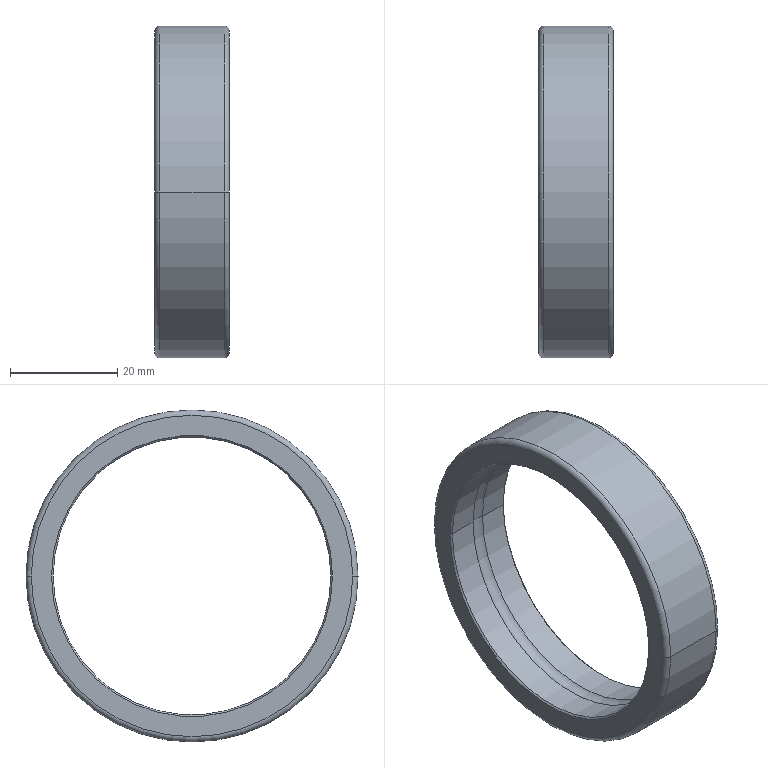Part | SolidWorks | 1 solid | 18 faces | box 14 x 62 x 62 mm | volume 12465 mm3 | cylinder 6 | torus 6 | cone 4 | plane 2 | commonest cylinder face diameters 51.875 x4 62 x2
STEP:
#1=CARTESIAN_POINT('',(0.3,-25.938,0.));
#2=VERTEX_POINT('',#1);
#3=CARTESIAN_POINT('',(0.,-26.238,0.));
#4=VERTEX_POINT('',#3);
#5=CARTESIAN_POINT('',(0.3,-25.938,0.));
#6=DIRECTION('',(-0.7071,-0.7071,0.));
#7=VECTOR('',#6,1000.);
#8=LINE('',#5,#7);
#9=EDGE_CURVE('',#2,#4,#8,.T.);
#10=ORIENTED_EDGE('',*,*,#9,.T.);
#11=CARTESIAN_POINT('',(0.,26.238,0.));
#12=VERTEX_POINT('',#11);
#13=CARTESIAN_POINT('',(0.,0.,0.));
#14=DIRECTION('',(-1.,0.,0.));
#15=DIRECTION('',(0.,-1.,0.));
#16=AXIS2_PLACEMENT_3D('',#13,#14,#15);
#17=CIRCLE('',#16,26.238);
#18=EDGE_CURVE('',#4,#12,#17,.T.);
#19=ORIENTED_EDGE('',*,*,#18,.T.);
#20=CARTESIAN_POINT('',(0.3,25.938,0.));
#21=VERTEX_POINT('',#20);
#22=CARTESIAN_POINT('',(0.3,25.938,0.));
#23=DIRECTION('',(-0.7071,0.7071,0.));
#24=VECTOR('',#23,1000.);
#25=LINE('',#22,#24);
#26=EDGE_CURVE('',#21,#12,#25,.T.);
#27=ORIENTED_EDGE('',*,*,#26,.F.);
#28=CARTESIAN_POINT('',(0.3,0.,0.));
#29=DIRECTION('',(-1.,0.,0.));
#30=DIRECTION('',(0.,-1.,0.));
#31=AXIS2_PLACEMENT_3D('',#28,#29,#30);
#32=CIRCLE('',#31,25.938);
#33=EDGE_CURVE('',#2,#21,#32,.T.);
#34=ORIENTED_EDGE('',*,*,#33,.F.);
#35=EDGE_LOOP('',(#10,#19,#27,#34));
#36=FACE_OUTER_BOUND('',#35,.T.);
#37=CARTESIAN_POINT('',(0.3753,0.,0.));
#38=DIRECTION('',(-1.,0.,0.));
#39=DIRECTION('',(0.,1.,0.));
#40=AXIS2_PLACEMENT_3D('',#37,#38,#39);
#41=CONICAL_SURFACE('',#40,25.862,0.7854);
#42=ADVANCED_FACE('',(#36),#41,.F.);
#43=CARTESIAN_POINT('',(13.7,-25.938,0.));
#44=VERTEX_POINT('',#43);
#45=CARTESIAN_POINT('',(8.25,-25.938,0.));
#46=VERTEX_POINT('',#45);
#47=CARTESIAN_POINT('',(13.7,-25.938,0.));
#48=DIRECTION('',(-1.,0.,0.));
#49=VECTOR('',#48,1000.);
#50=LINE('',#47,#49);
#51=EDGE_CURVE('',#44,#46,#50,.T.);
#52=ORIENTED_EDGE('',*,*,#51,.T.);
#53=CARTESIAN_POINT('',(8.25,25.938,0.));
#54=VERTEX_POINT('',#53);
#55=CARTESIAN_POINT('',(8.25,0.,0.));
#56=DIRECTION('',(-1.,0.,0.));
#57=DIRECTION('',(0.,-1.,0.));
#58=AXIS2_PLACEMENT_3D('',#55,#56,#57);
#59=CIRCLE('',#58,25.938);
#60=EDGE_CURVE('',#46,#54,#59,.T.);
#61=ORIENTED_EDGE('',*,*,#60,.T.);
#62=CARTESIAN_POINT('',(13.7,25.938,0.));
#63=VERTEX_POINT('',#62);
#64=CARTESIAN_POINT('',(13.7,25.938,0.));
#65=DIRECTION('',(-1.,0.,0.));
#66=VECTOR('',#65,1000.);
#67=LINE('',#64,#66);
#68=EDGE_CURVE('',#63,#54,#67,.T.);
#69=ORIENTED_EDGE('',*,*,#68,.F.);
#70=CARTESIAN_POINT('',(13.7,0.,0.));
#71=DIRECTION('',(1.,0.,0.));
#72=DIRECTION('',(0.,1.,0.));
#73=AXIS2_PLACEMENT_3D('',#70,#71,#72);
#74=CIRCLE('',#73,25.938);
#75=EDGE_CURVE('',#63,#44,#74,.T.);
#76=ORIENTED_EDGE('',*,*,#75,.T.);
#77=EDGE_LOOP('',(#52,#61,#69,#76));
#78=FACE_OUTER_BOUND('',#77,.T.);
#79=CARTESIAN_POINT('',(0.,0.,0.));
#80=DIRECTION('',(1.,0.,0.));
#81=DIRECTION('',(0.,-1.,0.));
#82=AXIS2_PLACEMENT_3D('',#79,#80,#81);
#83=CYLINDRICAL_SURFACE('',#82,25.938);
#84=ADVANCED_FACE('',(#78),#83,.F.);
#85=CARTESIAN_POINT('',(5.75,-25.938,0.));
#86=VERTEX_POINT('',#85);
#87=CARTESIAN_POINT('',(7.,-24.25,0.));
#88=DIRECTION('',(0.,0.,-1.));
#89=DIRECTION('',(0.5952,-0.8036,0.));
#90=AXIS2_PLACEMENT_3D('',#87,#88,#89);
#91=CIRCLE('',#90,2.1);
#92=EDGE_CURVE('',#46,#86,#91,.T.);
#93=ORIENTED_EDGE('',*,*,#92,.T.);
#94=CARTESIAN_POINT('',(5.75,25.938,0.));
#95=VERTEX_POINT('',#94);
#96=CARTESIAN_POINT('',(5.75,0.,0.));
#97=DIRECTION('',(1.,0.,0.));
#98=DIRECTION('',(0.,1.,0.));
#99=AXIS2_PLACEMENT_3D('',#96,#97,#98);
#100=CIRCLE('',#99,25.938);
#101=EDGE_CURVE('',#95,#86,#100,.T.);
#102=ORIENTED_EDGE('',*,*,#101,.F.);
#103=CARTESIAN_POINT('',(7.,24.25,0.));
#104=DIRECTION('',(0.,0.,1.));
#105=DIRECTION('',(0.,1.,0.));
#106=AXIS2_PLACEMENT_3D('',#103,#104,#105);
#107=CIRCLE('',#106,2.1);
#108=EDGE_CURVE('',#54,#95,#107,.T.);
#109=ORIENTED_EDGE('',*,*,#108,.F.);
#110=ORIENTED_EDGE('',*,*,#60,.F.);
#111=EDGE_LOOP('',(#93,#102,#109,#110));
#112=FACE_OUTER_BOUND('',#111,.T.);
#113=CARTESIAN_POINT('',(7.,0.,0.));
#114=DIRECTION('',(1.,0.,0.));
#115=DIRECTION('',(0.,-1.,0.));
#116=AXIS2_PLACEMENT_3D('',#113,#114,#115);
#117=TOROIDAL_SURFACE('',#116,24.25,2.1);
#118=ADVANCED_FACE('',(#112),#117,.F.);
#119=CARTESIAN_POINT('',(5.75,-25.938,0.));
#120=DIRECTION('',(-1.,0.,0.));
#121=VECTOR('',#120,1000.);
#122=LINE('',#119,#121);
#123=EDGE_CURVE('',#86,#2,#122,.T.);
#124=ORIENTED_EDGE('',*,*,#123,.T.);
#125=ORIENTED_EDGE('',*,*,#33,.T.);
#126=CARTESIAN_POINT('',(5.75,25.938,0.));
#127=DIRECTION('',(-1.,0.,0.));
#128=VECTOR('',#127,1000.);
#129=LINE('',#126,#128);
#130=EDGE_CURVE('',#95,#21,#129,.T.);
#131=ORIENTED_EDGE('',*,*,#130,.F.);
#132=ORIENTED_EDGE('',*,*,#101,.T.);
#133=EDGE_LOOP('',(#124,#125,#131,#132));
#134=FACE_OUTER_BOUND('',#133,.T.);
#135=CARTESIAN_POINT('',(0.,0.,0.));
#136=DIRECTION('',(1.,0.,0.));
#137=DIRECTION('',(0.,-1.,0.));
#138=AXIS2_PLACEMENT_3D('',#135,#136,#137);
#139=CYLINDRICAL_SURFACE('',#138,25.938);
#140=ADVANCED_FACE('',(#134),#139,.F.);
#141=ORIENTED_EDGE('',*,*,#123,.F.);
#142=CARTESIAN_POINT('',(5.75,0.,0.));
#143=DIRECTION('',(1.,0.,0.));
#144=DIRECTION('',(0.,-1.,0.));
#145=AXIS2_PLACEMENT_3D('',#142,#143,#144);
#146=CIRCLE('',#145,25.938);
#147=EDGE_CURVE('',#86,#95,#146,.T.);
#148=ORIENTED_EDGE('',*,*,#147,.T.);
#149=ORIENTED_EDGE('',*,*,#130,.T.);
#150=CARTESIAN_POINT('',(0.3,0.,0.));
#151=DIRECTION('',(-1.,0.,0.));
#152=DIRECTION('',(0.,1.,0.));
#153=AXIS2_PLACEMENT_3D('',#150,#151,#152);
#154=CIRCLE('',#153,25.938);
#155=EDGE_CURVE('',#21,#2,#154,.T.);
#156=ORIENTED_EDGE('',*,*,#155,.T.);
#157=EDGE_LOOP('',(#141,#148,#149,#156));
#158=FACE_OUTER_BOUND('',#157,.T.);
#159=CARTESIAN_POINT('',(0.,0.,0.));
#160=DIRECTION('',(1.,0.,0.));
#161=DIRECTION('',(0.,-1.,0.));
#162=AXIS2_PLACEMENT_3D('',#159,#160,#161);
#163=CYLINDRICAL_SURFACE('',#162,25.938);
#164=ADVANCED_FACE('',(#158),#163,.F.);
#165=ORIENTED_EDGE('',*,*,#147,.F.);
#166=ORIENTED_EDGE('',*,*,#92,.F.);
#167=CARTESIAN_POINT('',(8.25,0.,0.));
#168=DIRECTION('',(-1.,0.,0.));
#169=DIRECTION('',(0.,1.,0.));
#170=AXIS2_PLACEMENT_3D('',#167,#168,#169);
#171=CIRCLE('',#170,25.938);
#172=EDGE_CURVE('',#54,#46,#171,.T.);
#173=ORIENTED_EDGE('',*,*,#172,.F.);
#174=ORIENTED_EDGE('',*,*,#108,.T.);
#175=EDGE_LOOP('',(#165,#166,#173,#174));
#176=FACE_OUTER_BOUND('',#175,.T.);
#177=CARTESIAN_POINT('',(7.,0.,0.));
#178=DIRECTION('',(1.,0.,0.));
#179=DIRECTION('',(0.,-1.,0.));
#180=AXIS2_PLACEMENT_3D('',#177,#178,#179);
#181=TOROIDAL_SURFACE('',#180,24.25,2.1);
#182=ADVANCED_FACE('',(#176),#181,.F.);
#183=ORIENTED_EDGE('',*,*,#51,.F.);
#184=CARTESIAN_POINT('',(13.7,0.,0.));
#185=DIRECTION('',(1.,0.,0.));
#186=DIRECTION('',(0.,-1.,0.));
#187=AXIS2_PLACEMENT_3D('',#184,#185,#186);
#188=CIRCLE('',#187,25.938);
#189=EDGE_CURVE('',#44,#63,#188,.T.);
#190=ORIENTED_EDGE('',*,*,#189,.T.);
#191=ORIENTED_EDGE('',*,*,#68,.T.);
#192=ORIENTED_EDGE('',*,*,#172,.T.);
#193=EDGE_LOOP('',(#183,#190,#191,#192));
#194=FACE_OUTER_BOUND('',#193,.T.);
#195=CARTESIAN_POINT('',(0.,0.,0.));
#196=DIRECTION('',(1.,0.,0.));
#197=DIRECTION('',(0.,-1.,0.));
#198=AXIS2_PLACEMENT_3D('',#195,#196,#197);
#199=CYLINDRICAL_SURFACE('',#198,25.938);
#200=ADVANCED_FACE('',(#194),#199,.F.);
#201=CARTESIAN_POINT('',(14.,-26.238,0.));
#202=VERTEX_POINT('',#201);
#203=CARTESIAN_POINT('',(14.,-26.238,0.));
#204=DIRECTION('',(-0.7071,0.7071,0.));
#205=VECTOR('',#204,1000.);
#206=LINE('',#203,#205);
#207=EDGE_CURVE('',#202,#44,#206,.T.);
#208=ORIENTED_EDGE('',*,*,#207,.F.);
#209=CARTESIAN_POINT('',(14.,26.238,0.));
#210=VERTEX_POINT('',#209);
#211=CARTESIAN_POINT('',(14.,0.,0.));
#212=DIRECTION('',(1.,0.,0.));
#213=DIRECTION('',(0.,-1.,0.));
#214=AXIS2_PLACEMENT_3D('',#211,#212,#213);
#215=CIRCLE('',#214,26.238);
#216=EDGE_CURVE('',#202,#210,#215,.T.);
#217=ORIENTED_EDGE('',*,*,#216,.T.);
#218=CARTESIAN_POINT('',(14.,26.238,0.));
#219=DIRECTION('',(-0.7071,-0.7071,0.));
#220=VECTOR('',#219,1000.);
#221=LINE('',#218,#220);
#222=EDGE_CURVE('',#210,#63,#221,.T.);
#223=ORIENTED_EDGE('',*,*,#222,.T.);
#224=ORIENTED_EDGE('',*,*,#189,.F.);
#225=EDGE_LOOP('',(#208,#217,#223,#224));
#226=FACE_OUTER_BOUND('',#225,.T.);
#227=CARTESIAN_POINT('',(13.625,0.,0.));
#228=DIRECTION('',(1.,0.,0.));
#229=DIRECTION('',(0.,-1.,0.));
#230=AXIS2_PLACEMENT_3D('',#227,#228,#229);
#231=CONICAL_SURFACE('',#230,25.862,0.7854);
#232=ADVANCED_FACE('',(#226),#231,.F.);
#233=ORIENTED_EDGE('',*,*,#207,.T.);
#234=ORIENTED_EDGE('',*,*,#75,.F.);
#235=ORIENTED_EDGE('',*,*,#222,.F.);
#236=CARTESIAN_POINT('',(14.,0.,0.));
#237=DIRECTION('',(1.,0.,0.));
#238=DIRECTION('',(0.,1.,0.));
#239=AXIS2_PLACEMENT_3D('',#236,#237,#238);
#240=CIRCLE('',#239,26.238);
#241=EDGE_CURVE('',#210,#202,#240,.T.);
#242=ORIENTED_EDGE('',*,*,#241,.T.);
#243=EDGE_LOOP('',(#233,#234,#235,#242));
#244=FACE_OUTER_BOUND('',#243,.T.);
#245=CARTESIAN_POINT('',(13.625,0.,0.));
#246=DIRECTION('',(1.,0.,0.));
#247=DIRECTION('',(0.,-1.,0.));
#248=AXIS2_PLACEMENT_3D('',#245,#246,#247);
#249=CONICAL_SURFACE('',#248,25.862,0.7854);
#250=ADVANCED_FACE('',(#244),#249,.F.);
#251=CARTESIAN_POINT('',(1.,-31.,0.));
#252=VERTEX_POINT('',#251);
#253=CARTESIAN_POINT('',(13.,-31.,0.));
#254=VERTEX_POINT('',#253);
#255=CARTESIAN_POINT('',(1.,-31.,0.));
#256=DIRECTION('',(1.,0.,0.));
#257=VECTOR('',#256,1000.);
#258=LINE('',#255,#257);
#259=EDGE_CURVE('',#252,#254,#258,.T.);
#260=ORIENTED_EDGE('',*,*,#259,.T.);
#261=CARTESIAN_POINT('',(13.,31.,0.));
#262=VERTEX_POINT('',#261);
#263=CARTESIAN_POINT('',(13.,0.,0.));
#264=DIRECTION('',(-1.,0.,0.));
#265=DIRECTION('',(0.,-1.,0.));
#266=AXIS2_PLACEMENT_3D('',#263,#264,#265);
#267=CIRCLE('',#266,31.);
#268=EDGE_CURVE('',#254,#262,#267,.T.);
#269=ORIENTED_EDGE('',*,*,#268,.T.);
#270=CARTESIAN_POINT('',(1.,31.,0.));
#271=VERTEX_POINT('',#270);
#272=CARTESIAN_POINT('',(1.,31.,0.));
#273=DIRECTION('',(1.,0.,0.));
#274=VECTOR('',#273,1000.);
#275=LINE('',#272,#274);
#276=EDGE_CURVE('',#271,#262,#275,.T.);
#277=ORIENTED_EDGE('',*,*,#276,.F.);
#278=CARTESIAN_POINT('',(1.,0.,0.));
#279=DIRECTION('',(1.,0.,0.));
#280=DIRECTION('',(0.,1.,0.));
#281=AXIS2_PLACEMENT_3D('',#278,#279,#280);
#282=CIRCLE('',#281,31.);
#283=EDGE_CURVE('',#271,#252,#282,.T.);
#284=ORIENTED_EDGE('',*,*,#283,.T.);
#285=EDGE_LOOP('',(#260,#269,#277,#284));
#286=FACE_OUTER_BOUND('',#285,.T.);
#287=CARTESIAN_POINT('',(0.,0.,0.));
#288=DIRECTION('',(1.,0.,0.));
#289=DIRECTION('',(0.,-1.,0.));
#290=AXIS2_PLACEMENT_3D('',#287,#288,#289);
#291=CYLINDRICAL_SURFACE('',#290,31.);
#292=ADVANCED_FACE('',(#286),#291,.T.);
#293=CARTESIAN_POINT('',(14.,-30.,0.));
#294=VERTEX_POINT('',#293);
#295=CARTESIAN_POINT('',(13.,-30.,0.));
#296=DIRECTION('',(0.,0.,1.));
#297=DIRECTION('',(0.,-1.,0.));
#298=AXIS2_PLACEMENT_3D('',#295,#296,#297);
#299=CIRCLE('',#298,1.);
#300=EDGE_CURVE('',#254,#294,#299,.T.);
#301=ORIENTED_EDGE('',*,*,#300,.T.);
#302=CARTESIAN_POINT('',(14.,30.,0.));
#303=VERTEX_POINT('',#302);
#304=CARTESIAN_POINT('',(14.,0.,0.));
#305=DIRECTION('',(-1.,0.,0.));
#306=DIRECTION('',(0.,-1.,0.));
#307=AXIS2_PLACEMENT_3D('',#304,#305,#306);
#308=CIRCLE('',#307,30.);
#309=EDGE_CURVE('',#294,#303,#308,.T.);
#310=ORIENTED_EDGE('',*,*,#309,.T.);
#311=CARTESIAN_POINT('',(13.,30.,0.));
#312=DIRECTION('',(0.,0.,-1.));
#313=DIRECTION('',(0.,1.,0.));
#314=AXIS2_PLACEMENT_3D('',#311,#312,#313);
#315=CIRCLE('',#314,1.);
#316=EDGE_CURVE('',#262,#303,#315,.T.);
#317=ORIENTED_EDGE('',*,*,#316,.F.);
#318=ORIENTED_EDGE('',*,*,#268,.F.);
#319=EDGE_LOOP('',(#301,#310,#317,#318));
#320=FACE_OUTER_BOUND('',#319,.T.);
#321=CARTESIAN_POINT('',(13.,0.,0.));
#322=DIRECTION('',(1.,0.,0.));
#323=DIRECTION('',(0.,-1.,0.));
#324=AXIS2_PLACEMENT_3D('',#321,#322,#323);
#325=TOROIDAL_SURFACE('',#324,30.,1.);
#326=ADVANCED_FACE('',(#320),#325,.T.);
#327=ORIENTED_EDGE('',*,*,#216,.F.);
#328=ORIENTED_EDGE('',*,*,#241,.F.);
#329=EDGE_LOOP('',(#327,#328));
#330=FACE_BOUND('',#329,.T.);
#331=ORIENTED_EDGE('',*,*,#309,.F.);
#332=CARTESIAN_POINT('',(14.,0.,0.));
#333=DIRECTION('',(-1.,0.,0.));
#334=DIRECTION('',(0.,1.,0.));
#335=AXIS2_PLACEMENT_3D('',#332,#333,#334);
#336=CIRCLE('',#335,30.);
#337=EDGE_CURVE('',#303,#294,#336,.T.);
#338=ORIENTED_EDGE('',*,*,#337,.F.);
#339=EDGE_LOOP('',(#331,#338));
#340=FACE_OUTER_BOUND('',#339,.T.);
#341=CARTESIAN_POINT('',(14.,0.,0.));
#342=DIRECTION('',(1.,0.,0.));
#343=DIRECTION('',(0.,1.,0.));
#344=AXIS2_PLACEMENT_3D('',#341,#342,#343);
#345=PLANE('',#344);
#346=ADVANCED_FACE('',(#330,#340),#345,.T.);
#347=ORIENTED_EDGE('',*,*,#300,.F.);
#348=CARTESIAN_POINT('',(13.,0.,0.));
#349=DIRECTION('',(-1.,0.,0.));
#350=DIRECTION('',(0.,1.,0.));
#351=AXIS2_PLACEMENT_3D('',#348,#349,#350);
#352=CIRCLE('',#351,31.);
#353=EDGE_CURVE('',#262,#254,#352,.T.);
#354=ORIENTED_EDGE('',*,*,#353,.F.);
#355=ORIENTED_EDGE('',*,*,#316,.T.);
#356=ORIENTED_EDGE('',*,*,#337,.T.);
#357=EDGE_LOOP('',(#347,#354,#355,#356));
#358=FACE_OUTER_BOUND('',#357,.T.);
#359=CARTESIAN_POINT('',(13.,0.,0.));
#360=DIRECTION('',(1.,0.,0.));
#361=DIRECTION('',(0.,-1.,0.));
#362=AXIS2_PLACEMENT_3D('',#359,#360,#361);
#363=TOROIDAL_SURFACE('',#362,30.,1.);
#364=ADVANCED_FACE('',(#358),#363,.T.);
#365=ORIENTED_EDGE('',*,*,#259,.F.);
#366=CARTESIAN_POINT('',(1.,0.,0.));
#367=DIRECTION('',(1.,0.,0.));
#368=DIRECTION('',(0.,-1.,0.));
#369=AXIS2_PLACEMENT_3D('',#366,#367,#368);
#370=CIRCLE('',#369,31.);
#371=EDGE_CURVE('',#252,#271,#370,.T.);
#372=ORIENTED_EDGE('',*,*,#371,.T.);
#373=ORIENTED_EDGE('',*,*,#276,.T.);
#374=ORIENTED_EDGE('',*,*,#353,.T.);
#375=EDGE_LOOP('',(#365,#372,#373,#374));
#376=FACE_OUTER_BOUND('',#375,.T.);
#377=CARTESIAN_POINT('',(0.,0.,0.));
#378=DIRECTION('',(1.,0.,0.));
#379=DIRECTION('',(0.,-1.,0.));
#380=AXIS2_PLACEMENT_3D('',#377,#378,#379);
#381=CYLINDRICAL_SURFACE('',#380,31.);
#382=ADVANCED_FACE('',(#376),#381,.T.);
#383=CARTESIAN_POINT('',(0.,-30.,0.));
#384=VERTEX_POINT('',#383);
#385=CARTESIAN_POINT('',(1.,-30.,0.));
#386=DIRECTION('',(0.,0.,1.));
#387=DIRECTION('',(-1.,0.,0.));
#388=AXIS2_PLACEMENT_3D('',#385,#386,#387);
#389=CIRCLE('',#388,1.);
#390=EDGE_CURVE('',#384,#252,#389,.T.);
#391=ORIENTED_EDGE('',*,*,#390,.F.);
#392=CARTESIAN_POINT('',(0.,30.,0.));
#393=VERTEX_POINT('',#392);
#394=CARTESIAN_POINT('',(0.,0.,0.));
#395=DIRECTION('',(1.,0.,0.));
#396=DIRECTION('',(0.,-1.,0.));
#397=AXIS2_PLACEMENT_3D('',#394,#395,#396);
#398=CIRCLE('',#397,30.);
#399=EDGE_CURVE('',#384,#393,#398,.T.);
#400=ORIENTED_EDGE('',*,*,#399,.T.);
#401=CARTESIAN_POINT('',(1.,30.,0.));
#402=DIRECTION('',(0.,0.,-1.));
#403=DIRECTION('',(-1.,0.,0.));
#404=AXIS2_PLACEMENT_3D('',#401,#402,#403);
#405=CIRCLE('',#404,1.);
#406=EDGE_CURVE('',#393,#271,#405,.T.);
#407=ORIENTED_EDGE('',*,*,#406,.T.);
#408=ORIENTED_EDGE('',*,*,#371,.F.);
#409=EDGE_LOOP('',(#391,#400,#407,#408));
#410=FACE_OUTER_BOUND('',#409,.T.);
#411=CARTESIAN_POINT('',(1.,0.,0.));
#412=DIRECTION('',(1.,0.,0.));
#413=DIRECTION('',(0.,-1.,0.));
#414=AXIS2_PLACEMENT_3D('',#411,#412,#413);
#415=TOROIDAL_SURFACE('',#414,30.,1.);
#416=ADVANCED_FACE('',(#410),#415,.T.);
#417=ORIENTED_EDGE('',*,*,#390,.T.);
#418=ORIENTED_EDGE('',*,*,#283,.F.);
#419=ORIENTED_EDGE('',*,*,#406,.F.);
#420=CARTESIAN_POINT('',(0.,0.,0.));
#421=DIRECTION('',(1.,0.,0.));
#422=DIRECTION('',(0.,1.,0.));
#423=AXIS2_PLACEMENT_3D('',#420,#421,#422);
#424=CIRCLE('',#423,30.);
#425=EDGE_CURVE('',#393,#384,#424,.T.);
#426=ORIENTED_EDGE('',*,*,#425,.T.);
#427=EDGE_LOOP('',(#417,#418,#419,#426));
#428=FACE_OUTER_BOUND('',#427,.T.);
#429=CARTESIAN_POINT('',(1.,0.,0.));
#430=DIRECTION('',(1.,0.,0.));
#431=DIRECTION('',(0.,-1.,0.));
#432=AXIS2_PLACEMENT_3D('',#429,#430,#431);
#433=TOROIDAL_SURFACE('',#432,30.,1.);
#434=ADVANCED_FACE('',(#428),#433,.T.);
#435=ORIENTED_EDGE('',*,*,#18,.F.);
#436=CARTESIAN_POINT('',(0.,0.,0.));
#437=DIRECTION('',(-1.,0.,0.));
#438=DIRECTION('',(0.,1.,0.));
#439=AXIS2_PLACEMENT_3D('',#436,#437,#438);
#440=CIRCLE('',#439,26.238);
#441=EDGE_CURVE('',#12,#4,#440,.T.);
#442=ORIENTED_EDGE('',*,*,#441,.F.);
#443=EDGE_LOOP('',(#435,#442));
#444=FACE_BOUND('',#443,.T.);
#445=ORIENTED_EDGE('',*,*,#399,.F.);
#446=ORIENTED_EDGE('',*,*,#425,.F.);
#447=EDGE_LOOP('',(#445,#446));
#448=FACE_OUTER_BOUND('',#447,.T.);
#449=CARTESIAN_POINT('',(0.,0.,0.));
#450=DIRECTION('',(1.,0.,0.));
#451=DIRECTION('',(0.,1.,0.));
#452=AXIS2_PLACEMENT_3D('',#449,#450,#451);
#453=PLANE('',#452);
#454=ADVANCED_FACE('',(#444,#448),#453,.F.);
#455=ORIENTED_EDGE('',*,*,#9,.F.);
#456=ORIENTED_EDGE('',*,*,#155,.F.);
#457=ORIENTED_EDGE('',*,*,#26,.T.);
#458=ORIENTED_EDGE('',*,*,#441,.T.);
#459=EDGE_LOOP('',(#455,#456,#457,#458));
#460=FACE_OUTER_BOUND('',#459,.T.);
#461=CARTESIAN_POINT('',(0.3753,0.,0.));
#462=DIRECTION('',(-1.,0.,0.));
#463=DIRECTION('',(0.,1.,0.));
#464=AXIS2_PLACEMENT_3D('',#461,#462,#463);
#465=CONICAL_SURFACE('',#464,25.862,0.7854);
#466=ADVANCED_FACE('',(#460),#465,.F.);
#467=CLOSED_SHELL('',(#42,#84,#118,#140,#164,#182,#200,#232,#250,#292,#326,#346,#364,#382,#416,#434,#454,#466));
#468=MANIFOLD_SOLID_BREP('',#467);
#469=CARTESIAN_POINT('',(0.,0.,0.));
#470=DIRECTION('',(0.,0.,1.));
#471=DIRECTION('',(1.,0.,0.));
#472=AXIS2_PLACEMENT_3D('',#469,#470,#471);
#473=(LENGTH_UNIT()NAMED_UNIT(*)SI_UNIT(.MILLI.,.METRE.));
#474=UNCERTAINTY_MEASURE_WITH_UNIT(LENGTH_MEASURE(0.00001),#473,'','');
#475=(NAMED_UNIT(*)PLANE_ANGLE_UNIT()SI_UNIT($,.RADIAN.));
#476=(NAMED_UNIT(*)SI_UNIT($,.STERADIAN.)SOLID_ANGLE_UNIT());
#477=(GEOMETRIC_REPRESENTATION_CONTEXT(3)GLOBAL_UNCERTAINTY_ASSIGNED_CONTEXT((#474))GLOBAL_UNIT_ASSIGNED_CONTEXT((#473,#475,#476))REPRESENTATION_CONTEXT('',''));
#478=ADVANCED_BREP_SHAPE_REPRESENTATION('',(#468,#472),#477);